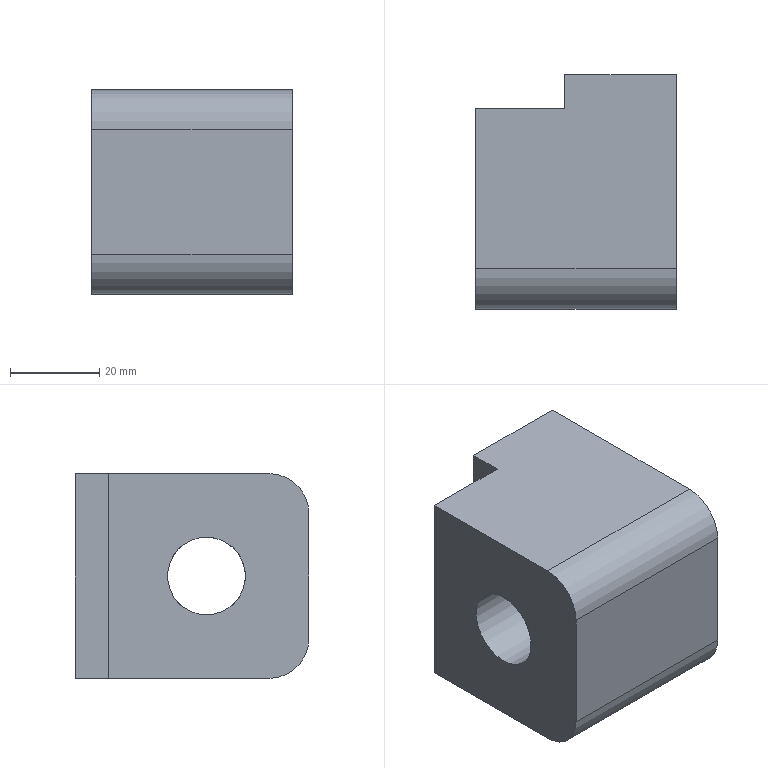Part | STEP file | solid 74 | 1 solid | 13 faces | box 45 x 52.5 x 46 mm | volume 85031 mm3 | plane 7 | cylinder 4 | spline 2 | commonest cylinder face diameters 18 x2 17.5 x1 26 x1